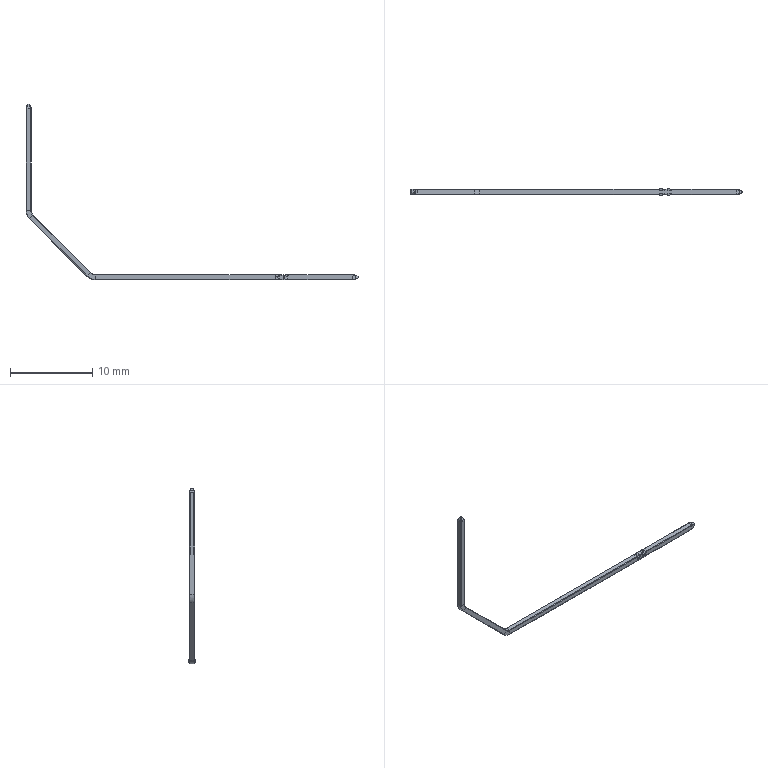Part | NX | features BREP 1 | 1 solid | 222 faces | box 40.315 x 0.8779 x 21.316 mm | volume 21.95 mm3 | cylinder 92 | plane 78 | torus 28 | sphere 20 | spline 4 | commonest cylinder face diameters 0.1 x32 0.09 x28 0.2 x12 2.01 x8 1 x4 2 x4